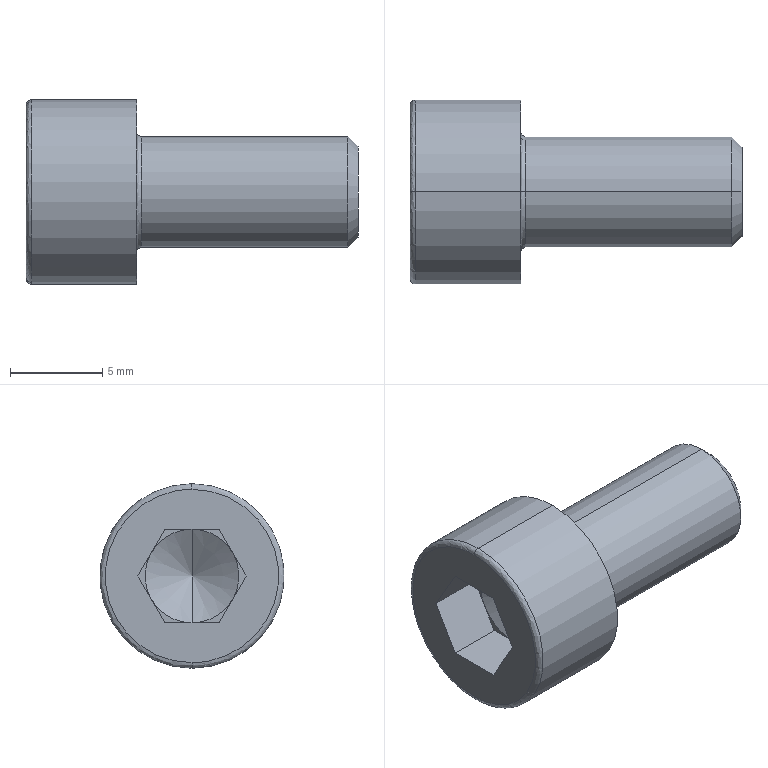Part | STEP file | PN_0071_default | 1 solid | 27 faces | box 18 x 10 x 10 mm | volume 730.412 mm3 | plane 15 | spline 4 | cylinder 4 | cone 4 | commonest cylinder face diameters 6 x2 10 x2